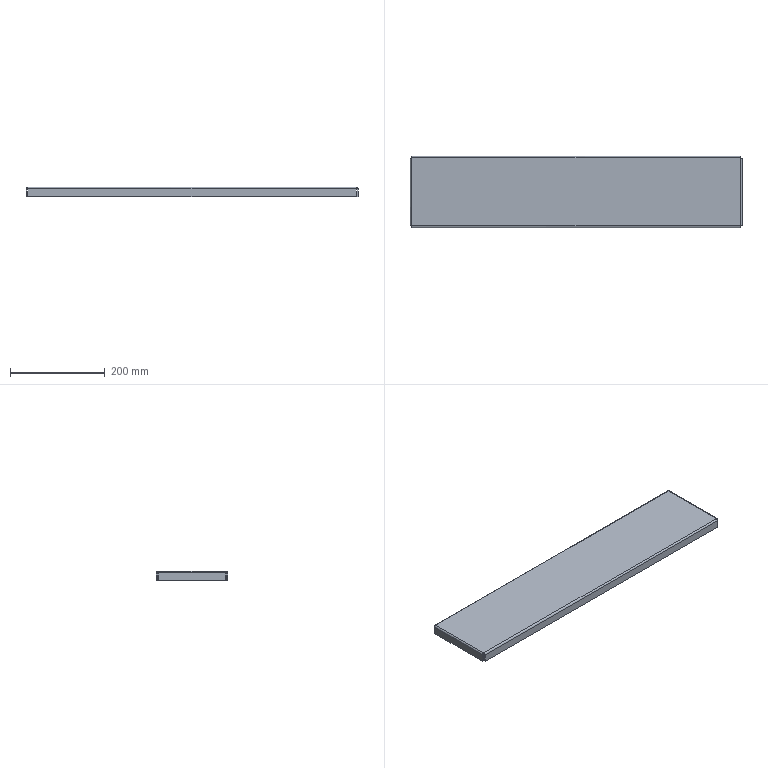Part | STEP file | PN_0053 top 304 stair tread 2_Default<As Machined> | 1 solid | 38 faces | box 700 x 150 x 20 mm | volume 396167 mm3 | plane 22 | spline 8 | cylinder 8 | commonest cylinder face diameters 0.6 x4 6.6 x4